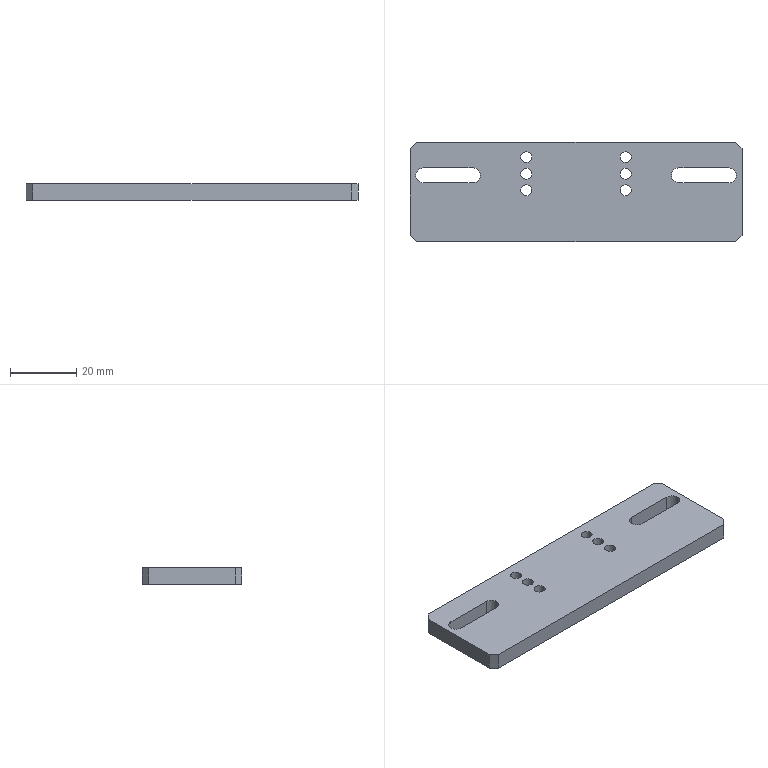Part | STEP file | 11-FG-SZ01611 | 1 solid | 32 faces | box 100 x 30 x 5 mm | volume 13869 mm3 | cylinder 18 | plane 14 | commonest cylinder face diameters 3.3 x12 4.5 x6
STEP:
#1=CARTESIAN_POINT('',(-28.75,5.,0.));
#2=VERTEX_POINT('',#1);
#3=CARTESIAN_POINT('',(-31.,7.25,0.));
#4=VERTEX_POINT('',#3);
#5=CARTESIAN_POINT('',(-31.,5.,0.));
#6=DIRECTION('',(0.,0.,1.));
#7=DIRECTION('',(1.,0.,0.));
#8=AXIS2_PLACEMENT_3D('',#5,#6,#7);
#9=CIRCLE('',#8,2.25);
#10=EDGE_CURVE('',#2,#4,#9,.T.);
#11=ORIENTED_EDGE('',*,*,#10,.F.);
#12=CARTESIAN_POINT('',(-28.75,5.,5.));
#13=VERTEX_POINT('',#12);
#14=CARTESIAN_POINT('',(-28.75,5.,-39.));
#15=DIRECTION('',(0.,0.,1.));
#16=VECTOR('',#15,1000.);
#17=LINE('',#14,#16);
#18=EDGE_CURVE('',#2,#13,#17,.T.);
#19=ORIENTED_EDGE('',*,*,#18,.T.);
#20=CARTESIAN_POINT('',(-31.,7.25,5.));
#21=VERTEX_POINT('',#20);
#22=CARTESIAN_POINT('',(-31.,5.,5.));
#23=DIRECTION('',(0.,0.,1.));
#24=DIRECTION('',(-1.,0.,0.));
#25=AXIS2_PLACEMENT_3D('',#22,#23,#24);
#26=CIRCLE('',#25,2.25);
#27=EDGE_CURVE('',#13,#21,#26,.T.);
#28=ORIENTED_EDGE('',*,*,#27,.T.);
#29=CARTESIAN_POINT('',(-31.,7.25,-39.));
#30=DIRECTION('',(0.,0.,1.));
#31=VECTOR('',#30,1000.);
#32=LINE('',#29,#31);
#33=EDGE_CURVE('',#4,#21,#32,.T.);
#34=ORIENTED_EDGE('',*,*,#33,.F.);
#35=EDGE_LOOP('',(#11,#19,#28,#34));
#36=FACE_OUTER_BOUND('',#35,.T.);
#37=CARTESIAN_POINT('',(-31.,5.,-39.));
#38=DIRECTION('',(0.,0.,1.));
#39=DIRECTION('',(1.,0.,0.));
#40=AXIS2_PLACEMENT_3D('',#37,#38,#39);
#41=CYLINDRICAL_SURFACE('',#40,2.25);
#42=ADVANCED_FACE('',(#36),#41,.F.);
#43=CARTESIAN_POINT('',(48.25,5.,0.));
#44=VERTEX_POINT('',#43);
#45=CARTESIAN_POINT('',(46.,7.25,0.));
#46=VERTEX_POINT('',#45);
#47=CARTESIAN_POINT('',(46.,5.,0.));
#48=DIRECTION('',(0.,0.,1.));
#49=DIRECTION('',(1.,0.,0.));
#50=AXIS2_PLACEMENT_3D('',#47,#48,#49);
#51=CIRCLE('',#50,2.25);
#52=EDGE_CURVE('',#44,#46,#51,.T.);
#53=ORIENTED_EDGE('',*,*,#52,.F.);
#54=CARTESIAN_POINT('',(48.25,5.,5.));
#55=VERTEX_POINT('',#54);
#56=CARTESIAN_POINT('',(48.25,5.,-39.));
#57=DIRECTION('',(0.,0.,1.));
#58=VECTOR('',#57,1000.);
#59=LINE('',#56,#58);
#60=EDGE_CURVE('',#44,#55,#59,.T.);
#61=ORIENTED_EDGE('',*,*,#60,.T.);
#62=CARTESIAN_POINT('',(46.,7.25,5.));
#63=VERTEX_POINT('',#62);
#64=CARTESIAN_POINT('',(46.,5.,5.));
#65=DIRECTION('',(0.,0.,1.));
#66=DIRECTION('',(1.,0.,0.));
#67=AXIS2_PLACEMENT_3D('',#64,#65,#66);
#68=CIRCLE('',#67,2.25);
#69=EDGE_CURVE('',#55,#63,#68,.T.);
#70=ORIENTED_EDGE('',*,*,#69,.T.);
#71=CARTESIAN_POINT('',(46.,7.25,-39.));
#72=DIRECTION('',(0.,0.,1.));
#73=VECTOR('',#72,1000.);
#74=LINE('',#71,#73);
#75=EDGE_CURVE('',#46,#63,#74,.T.);
#76=ORIENTED_EDGE('',*,*,#75,.F.);
#77=EDGE_LOOP('',(#53,#61,#70,#76));
#78=FACE_OUTER_BOUND('',#77,.T.);
#79=CARTESIAN_POINT('',(46.,5.,-39.));
#80=DIRECTION('',(0.,0.,1.));
#81=DIRECTION('',(1.,0.,0.));
#82=AXIS2_PLACEMENT_3D('',#79,#80,#81);
#83=CYLINDRICAL_SURFACE('',#82,2.25);
#84=ADVANCED_FACE('',(#78),#83,.F.);
#85=CARTESIAN_POINT('',(13.35,10.5,0.));
#86=VERTEX_POINT('',#85);
#87=CARTESIAN_POINT('',(16.65,10.5,0.));
#88=VERTEX_POINT('',#87);
#89=CARTESIAN_POINT('',(15.,10.5,0.));
#90=DIRECTION('',(0.,0.,1.));
#91=DIRECTION('',(1.,0.,0.));
#92=AXIS2_PLACEMENT_3D('',#89,#90,#91);
#93=CIRCLE('',#92,1.65);
#94=EDGE_CURVE('',#86,#88,#93,.T.);
#95=ORIENTED_EDGE('',*,*,#94,.F.);
#96=CARTESIAN_POINT('',(13.35,10.5,5.));
#97=VERTEX_POINT('',#96);
#98=CARTESIAN_POINT('',(13.35,10.5,5.));
#99=DIRECTION('',(0.,0.,1.));
#100=VECTOR('',#99,1000.);
#101=LINE('',#98,#100);
#102=EDGE_CURVE('',#86,#97,#101,.T.);
#103=ORIENTED_EDGE('',*,*,#102,.T.);
#104=CARTESIAN_POINT('',(16.65,10.5,5.));
#105=VERTEX_POINT('',#104);
#106=CARTESIAN_POINT('',(15.,10.5,5.));
#107=DIRECTION('',(0.,0.,1.));
#108=DIRECTION('',(1.,0.,0.));
#109=AXIS2_PLACEMENT_3D('',#106,#107,#108);
#110=CIRCLE('',#109,1.65);
#111=EDGE_CURVE('',#97,#105,#110,.T.);
#112=ORIENTED_EDGE('',*,*,#111,.T.);
#113=CARTESIAN_POINT('',(16.65,10.5,5.));
#114=DIRECTION('',(0.,0.,1.));
#115=VECTOR('',#114,1000.);
#116=LINE('',#113,#115);
#117=EDGE_CURVE('',#88,#105,#116,.T.);
#118=ORIENTED_EDGE('',*,*,#117,.F.);
#119=EDGE_LOOP('',(#95,#103,#112,#118));
#120=FACE_OUTER_BOUND('',#119,.T.);
#121=CARTESIAN_POINT('',(15.,10.5,5.));
#122=DIRECTION('',(0.,0.,1.));
#123=DIRECTION('',(1.,0.,0.));
#124=AXIS2_PLACEMENT_3D('',#121,#122,#123);
#125=CYLINDRICAL_SURFACE('',#124,1.65);
#126=ADVANCED_FACE('',(#120),#125,.F.);
#127=CARTESIAN_POINT('',(-16.65,10.5,0.));
#128=VERTEX_POINT('',#127);
#129=CARTESIAN_POINT('',(-13.35,10.5,0.));
#130=VERTEX_POINT('',#129);
#131=CARTESIAN_POINT('',(-15.,10.5,0.));
#132=DIRECTION('',(0.,0.,1.));
#133=DIRECTION('',(1.,0.,0.));
#134=AXIS2_PLACEMENT_3D('',#131,#132,#133);
#135=CIRCLE('',#134,1.65);
#136=EDGE_CURVE('',#128,#130,#135,.T.);
#137=ORIENTED_EDGE('',*,*,#136,.F.);
#138=CARTESIAN_POINT('',(-16.65,10.5,5.));
#139=VERTEX_POINT('',#138);
#140=CARTESIAN_POINT('',(-16.65,10.5,5.));
#141=DIRECTION('',(0.,0.,1.));
#142=VECTOR('',#141,1000.);
#143=LINE('',#140,#142);
#144=EDGE_CURVE('',#128,#139,#143,.T.);
#145=ORIENTED_EDGE('',*,*,#144,.T.);
#146=CARTESIAN_POINT('',(-13.35,10.5,5.));
#147=VERTEX_POINT('',#146);
#148=CARTESIAN_POINT('',(-15.,10.5,5.));
#149=DIRECTION('',(0.,0.,1.));
#150=DIRECTION('',(1.,0.,0.));
#151=AXIS2_PLACEMENT_3D('',#148,#149,#150);
#152=CIRCLE('',#151,1.65);
#153=EDGE_CURVE('',#139,#147,#152,.T.);
#154=ORIENTED_EDGE('',*,*,#153,.T.);
#155=CARTESIAN_POINT('',(-13.35,10.5,5.));
#156=DIRECTION('',(0.,0.,1.));
#157=VECTOR('',#156,1000.);
#158=LINE('',#155,#157);
#159=EDGE_CURVE('',#130,#147,#158,.T.);
#160=ORIENTED_EDGE('',*,*,#159,.F.);
#161=EDGE_LOOP('',(#137,#145,#154,#160));
#162=FACE_OUTER_BOUND('',#161,.T.);
#163=CARTESIAN_POINT('',(-15.,10.5,5.));
#164=DIRECTION('',(0.,0.,1.));
#165=DIRECTION('',(1.,0.,0.));
#166=AXIS2_PLACEMENT_3D('',#163,#164,#165);
#167=CYLINDRICAL_SURFACE('',#166,1.65);
#168=ADVANCED_FACE('',(#162),#167,.F.);
#169=CARTESIAN_POINT('',(13.35,5.5,0.));
#170=VERTEX_POINT('',#169);
#171=CARTESIAN_POINT('',(16.65,5.5,0.));
#172=VERTEX_POINT('',#171);
#173=CARTESIAN_POINT('',(15.,5.5,0.));
#174=DIRECTION('',(0.,0.,1.));
#175=DIRECTION('',(1.,0.,0.));
#176=AXIS2_PLACEMENT_3D('',#173,#174,#175);
#177=CIRCLE('',#176,1.65);
#178=EDGE_CURVE('',#170,#172,#177,.T.);
#179=ORIENTED_EDGE('',*,*,#178,.F.);
#180=CARTESIAN_POINT('',(13.35,5.5,5.));
#181=VERTEX_POINT('',#180);
#182=CARTESIAN_POINT('',(13.35,5.5,5.));
#183=DIRECTION('',(0.,0.,1.));
#184=VECTOR('',#183,1000.);
#185=LINE('',#182,#184);
#186=EDGE_CURVE('',#170,#181,#185,.T.);
#187=ORIENTED_EDGE('',*,*,#186,.T.);
#188=CARTESIAN_POINT('',(16.65,5.5,5.));
#189=VERTEX_POINT('',#188);
#190=CARTESIAN_POINT('',(15.,5.5,5.));
#191=DIRECTION('',(0.,0.,1.));
#192=DIRECTION('',(1.,0.,0.));
#193=AXIS2_PLACEMENT_3D('',#190,#191,#192);
#194=CIRCLE('',#193,1.65);
#195=EDGE_CURVE('',#181,#189,#194,.T.);
#196=ORIENTED_EDGE('',*,*,#195,.T.);
#197=CARTESIAN_POINT('',(16.65,5.5,5.));
#198=DIRECTION('',(0.,0.,1.));
#199=VECTOR('',#198,1000.);
#200=LINE('',#197,#199);
#201=EDGE_CURVE('',#172,#189,#200,.T.);
#202=ORIENTED_EDGE('',*,*,#201,.F.);
#203=EDGE_LOOP('',(#179,#187,#196,#202));
#204=FACE_OUTER_BOUND('',#203,.T.);
#205=CARTESIAN_POINT('',(15.,5.5,5.));
#206=DIRECTION('',(0.,0.,1.));
#207=DIRECTION('',(1.,0.,0.));
#208=AXIS2_PLACEMENT_3D('',#205,#206,#207);
#209=CYLINDRICAL_SURFACE('',#208,1.65);
#210=ADVANCED_FACE('',(#204),#209,.F.);
#211=CARTESIAN_POINT('',(-16.65,5.5,0.));
#212=VERTEX_POINT('',#211);
#213=CARTESIAN_POINT('',(-13.35,5.5,0.));
#214=VERTEX_POINT('',#213);
#215=CARTESIAN_POINT('',(-15.,5.5,0.));
#216=DIRECTION('',(0.,0.,1.));
#217=DIRECTION('',(1.,0.,0.));
#218=AXIS2_PLACEMENT_3D('',#215,#216,#217);
#219=CIRCLE('',#218,1.65);
#220=EDGE_CURVE('',#212,#214,#219,.T.);
#221=ORIENTED_EDGE('',*,*,#220,.F.);
#222=CARTESIAN_POINT('',(-16.65,5.5,5.));
#223=VERTEX_POINT('',#222);
#224=CARTESIAN_POINT('',(-16.65,5.5,5.));
#225=DIRECTION('',(0.,0.,1.));
#226=VECTOR('',#225,1000.);
#227=LINE('',#224,#226);
#228=EDGE_CURVE('',#212,#223,#227,.T.);
#229=ORIENTED_EDGE('',*,*,#228,.T.);
#230=CARTESIAN_POINT('',(-13.35,5.5,5.));
#231=VERTEX_POINT('',#230);
#232=CARTESIAN_POINT('',(-15.,5.5,5.));
#233=DIRECTION('',(0.,0.,1.));
#234=DIRECTION('',(1.,0.,0.));
#235=AXIS2_PLACEMENT_3D('',#232,#233,#234);
#236=CIRCLE('',#235,1.65);
#237=EDGE_CURVE('',#223,#231,#236,.T.);
#238=ORIENTED_EDGE('',*,*,#237,.T.);
#239=CARTESIAN_POINT('',(-13.35,5.5,5.));
#240=DIRECTION('',(0.,0.,1.));
#241=VECTOR('',#240,1000.);
#242=LINE('',#239,#241);
#243=EDGE_CURVE('',#214,#231,#242,.T.);
#244=ORIENTED_EDGE('',*,*,#243,.F.);
#245=EDGE_LOOP('',(#221,#229,#238,#244));
#246=FACE_OUTER_BOUND('',#245,.T.);
#247=CARTESIAN_POINT('',(-15.,5.5,5.));
#248=DIRECTION('',(0.,0.,1.));
#249=DIRECTION('',(1.,0.,0.));
#250=AXIS2_PLACEMENT_3D('',#247,#248,#249);
#251=CYLINDRICAL_SURFACE('',#250,1.65);
#252=ADVANCED_FACE('',(#246),#251,.F.);
#253=CARTESIAN_POINT('',(-16.65,0.5,0.));
#254=VERTEX_POINT('',#253);
#255=CARTESIAN_POINT('',(-13.35,0.5,0.));
#256=VERTEX_POINT('',#255);
#257=CARTESIAN_POINT('',(-15.,0.5,0.));
#258=DIRECTION('',(0.,0.,1.));
#259=DIRECTION('',(1.,0.,0.));
#260=AXIS2_PLACEMENT_3D('',#257,#258,#259);
#261=CIRCLE('',#260,1.65);
#262=EDGE_CURVE('',#254,#256,#261,.T.);
#263=ORIENTED_EDGE('',*,*,#262,.F.);
#264=CARTESIAN_POINT('',(-16.65,0.5,5.));
#265=VERTEX_POINT('',#264);
#266=CARTESIAN_POINT('',(-16.65,0.5,5.));
#267=DIRECTION('',(0.,0.,1.));
#268=VECTOR('',#267,1000.);
#269=LINE('',#266,#268);
#270=EDGE_CURVE('',#254,#265,#269,.T.);
#271=ORIENTED_EDGE('',*,*,#270,.T.);
#272=CARTESIAN_POINT('',(-13.35,0.5,5.));
#273=VERTEX_POINT('',#272);
#274=CARTESIAN_POINT('',(-15.,0.5,5.));
#275=DIRECTION('',(0.,0.,1.));
#276=DIRECTION('',(1.,0.,0.));
#277=AXIS2_PLACEMENT_3D('',#274,#275,#276);
#278=CIRCLE('',#277,1.65);
#279=EDGE_CURVE('',#265,#273,#278,.T.);
#280=ORIENTED_EDGE('',*,*,#279,.T.);
#281=CARTESIAN_POINT('',(-13.35,0.5,5.));
#282=DIRECTION('',(0.,0.,1.));
#283=VECTOR('',#282,1000.);
#284=LINE('',#281,#283);
#285=EDGE_CURVE('',#256,#273,#284,.T.);
#286=ORIENTED_EDGE('',*,*,#285,.F.);
#287=EDGE_LOOP('',(#263,#271,#280,#286));
#288=FACE_OUTER_BOUND('',#287,.T.);
#289=CARTESIAN_POINT('',(-15.,0.5,5.));
#290=DIRECTION('',(0.,0.,1.));
#291=DIRECTION('',(1.,0.,0.));
#292=AXIS2_PLACEMENT_3D('',#289,#290,#291);
#293=CYLINDRICAL_SURFACE('',#292,1.65);
#294=ADVANCED_FACE('',(#288),#293,.F.);
#295=CARTESIAN_POINT('',(13.35,0.5,0.));
#296=VERTEX_POINT('',#295);
#297=CARTESIAN_POINT('',(16.65,0.5,0.));
#298=VERTEX_POINT('',#297);
#299=CARTESIAN_POINT('',(15.,0.5,0.));
#300=DIRECTION('',(0.,0.,1.));
#301=DIRECTION('',(1.,0.,0.));
#302=AXIS2_PLACEMENT_3D('',#299,#300,#301);
#303=CIRCLE('',#302,1.65);
#304=EDGE_CURVE('',#296,#298,#303,.T.);
#305=ORIENTED_EDGE('',*,*,#304,.F.);
#306=CARTESIAN_POINT('',(13.35,0.5,5.));
#307=VERTEX_POINT('',#306);
#308=CARTESIAN_POINT('',(13.35,0.5,5.));
#309=DIRECTION('',(0.,0.,1.));
#310=VECTOR('',#309,1000.);
#311=LINE('',#308,#310);
#312=EDGE_CURVE('',#296,#307,#311,.T.);
#313=ORIENTED_EDGE('',*,*,#312,.T.);
#314=CARTESIAN_POINT('',(16.65,0.5,5.));
#315=VERTEX_POINT('',#314);
#316=CARTESIAN_POINT('',(15.,0.5,5.));
#317=DIRECTION('',(0.,0.,1.));
#318=DIRECTION('',(1.,0.,0.));
#319=AXIS2_PLACEMENT_3D('',#316,#317,#318);
#320=CIRCLE('',#319,1.65);
#321=EDGE_CURVE('',#307,#315,#320,.T.);
#322=ORIENTED_EDGE('',*,*,#321,.T.);
#323=CARTESIAN_POINT('',(16.65,0.5,5.));
#324=DIRECTION('',(0.,0.,1.));
#325=VECTOR('',#324,1000.);
#326=LINE('',#323,#325);
#327=EDGE_CURVE('',#298,#315,#326,.T.);
#328=ORIENTED_EDGE('',*,*,#327,.F.);
#329=EDGE_LOOP('',(#305,#313,#322,#328));
#330=FACE_OUTER_BOUND('',#329,.T.);
#331=CARTESIAN_POINT('',(15.,0.5,5.));
#332=DIRECTION('',(0.,0.,1.));
#333=DIRECTION('',(1.,0.,0.));
#334=AXIS2_PLACEMENT_3D('',#331,#332,#333);
#335=CYLINDRICAL_SURFACE('',#334,1.65);
#336=ADVANCED_FACE('',(#330),#335,.F.);
#337=CARTESIAN_POINT('',(50.,-13.,5.));
#338=VERTEX_POINT('',#337);
#339=CARTESIAN_POINT('',(50.,13.,5.));
#340=VERTEX_POINT('',#339);
#341=CARTESIAN_POINT('',(50.,15.,5.));
#342=DIRECTION('',(0.,1.,0.));
#343=VECTOR('',#342,1000.);
#344=LINE('',#341,#343);
#345=EDGE_CURVE('',#338,#340,#344,.T.);
#346=ORIENTED_EDGE('',*,*,#345,.F.);
#347=CARTESIAN_POINT('',(50.,-13.,0.));
#348=VERTEX_POINT('',#347);
#349=CARTESIAN_POINT('',(50.,-13.,5.));
#350=DIRECTION('',(0.,0.,-1.));
#351=VECTOR('',#350,1000.);
#352=LINE('',#349,#351);
#353=EDGE_CURVE('',#338,#348,#352,.T.);
#354=ORIENTED_EDGE('',*,*,#353,.T.);
#355=CARTESIAN_POINT('',(50.,13.,0.));
#356=VERTEX_POINT('',#355);
#357=CARTESIAN_POINT('',(50.,15.,0.));
#358=DIRECTION('',(0.,1.,0.));
#359=VECTOR('',#358,1000.);
#360=LINE('',#357,#359);
#361=EDGE_CURVE('',#348,#356,#360,.T.);
#362=ORIENTED_EDGE('',*,*,#361,.T.);
#363=CARTESIAN_POINT('',(50.,13.,5.));
#364=DIRECTION('',(0.,0.,1.));
#365=VECTOR('',#364,1000.);
#366=LINE('',#363,#365);
#367=EDGE_CURVE('',#356,#340,#366,.T.);
#368=ORIENTED_EDGE('',*,*,#367,.T.);
#369=EDGE_LOOP('',(#346,#354,#362,#368));
#370=FACE_OUTER_BOUND('',#369,.T.);
#371=CARTESIAN_POINT('',(50.,15.,5.));
#372=DIRECTION('',(-1.,0.,0.));
#373=DIRECTION('',(0.,-1.,0.));
#374=AXIS2_PLACEMENT_3D('',#371,#372,#373);
#375=PLANE('',#374);
#376=ADVANCED_FACE('',(#370),#375,.F.);
#377=CARTESIAN_POINT('',(48.,15.,0.));
#378=VERTEX_POINT('',#377);
#379=CARTESIAN_POINT('',(-48.,15.,0.));
#380=VERTEX_POINT('',#379);
#381=CARTESIAN_POINT('',(-50.,15.,0.));
#382=DIRECTION('',(-1.,0.,0.));
#383=VECTOR('',#382,1000.);
#384=LINE('',#381,#383);
#385=EDGE_CURVE('',#378,#380,#384,.T.);
#386=ORIENTED_EDGE('',*,*,#385,.T.);
#387=CARTESIAN_POINT('',(-48.,15.,5.));
#388=VERTEX_POINT('',#387);
#389=CARTESIAN_POINT('',(-48.,15.,5.));
#390=DIRECTION('',(0.,0.,1.));
#391=VECTOR('',#390,1000.);
#392=LINE('',#389,#391);
#393=EDGE_CURVE('',#380,#388,#392,.T.);
#394=ORIENTED_EDGE('',*,*,#393,.T.);
#395=CARTESIAN_POINT('',(48.,15.,5.));
#396=VERTEX_POINT('',#395);
#397=CARTESIAN_POINT('',(-50.,15.,5.));
#398=DIRECTION('',(-1.,0.,0.));
#399=VECTOR('',#398,1000.);
#400=LINE('',#397,#399);
#401=EDGE_CURVE('',#396,#388,#400,.T.);
#402=ORIENTED_EDGE('',*,*,#401,.F.);
#403=CARTESIAN_POINT('',(48.,15.,5.));
#404=DIRECTION('',(0.,0.,-1.));
#405=VECTOR('',#404,1000.);
#406=LINE('',#403,#405);
#407=EDGE_CURVE('',#396,#378,#406,.T.);
#408=ORIENTED_EDGE('',*,*,#407,.T.);
#409=EDGE_LOOP('',(#386,#394,#402,#408));
#410=FACE_OUTER_BOUND('',#409,.T.);
#411=CARTESIAN_POINT('',(-50.,15.,5.));
#412=DIRECTION('',(0.,-1.,0.));
#413=DIRECTION('',(0.,0.,-1.));
#414=AXIS2_PLACEMENT_3D('',#411,#412,#413);
#415=PLANE('',#414);
#416=ADVANCED_FACE('',(#410),#415,.F.);
#417=CARTESIAN_POINT('',(-50.,13.,0.));
#418=VERTEX_POINT('',#417);
#419=CARTESIAN_POINT('',(-50.,-13.,0.));
#420=VERTEX_POINT('',#419);
#421=CARTESIAN_POINT('',(-50.,15.,0.));
#422=DIRECTION('',(0.,-1.,0.));
#423=VECTOR('',#422,1000.);
#424=LINE('',#421,#423);
#425=EDGE_CURVE('',#418,#420,#424,.T.);
#426=ORIENTED_EDGE('',*,*,#425,.T.);
#427=CARTESIAN_POINT('',(-50.,-13.,5.));
#428=VERTEX_POINT('',#427);
#429=CARTESIAN_POINT('',(-50.,-13.,5.));
#430=DIRECTION('',(0.,0.,1.));
#431=VECTOR('',#430,1000.);
#432=LINE('',#429,#431);
#433=EDGE_CURVE('',#420,#428,#432,.T.);
#434=ORIENTED_EDGE('',*,*,#433,.T.);
#435=CARTESIAN_POINT('',(-50.,13.,5.));
#436=VERTEX_POINT('',#435);
#437=CARTESIAN_POINT('',(-50.,15.,5.));
#438=DIRECTION('',(0.,-1.,0.));
#439=VECTOR('',#438,1000.);
#440=LINE('',#437,#439);
#441=EDGE_CURVE('',#436,#428,#440,.T.);
#442=ORIENTED_EDGE('',*,*,#441,.F.);
#443=CARTESIAN_POINT('',(-50.,13.,5.));
#444=DIRECTION('',(0.,0.,-1.));
#445=VECTOR('',#444,1000.);
#446=LINE('',#443,#445);
#447=EDGE_CURVE('',#436,#418,#446,.T.);
#448=ORIENTED_EDGE('',*,*,#447,.T.);
#449=EDGE_LOOP('',(#426,#434,#442,#448));
#450=FACE_OUTER_BOUND('',#449,.T.);
#451=CARTESIAN_POINT('',(-50.,15.,5.));
#452=DIRECTION('',(1.,0.,0.));
#453=DIRECTION('',(0.,0.,-1.));
#454=AXIS2_PLACEMENT_3D('',#451,#452,#453);
#455=PLANE('',#454);
#456=ADVANCED_FACE('',(#450),#455,.F.);
#457=CARTESIAN_POINT('',(-48.,-15.,5.));
#458=VERTEX_POINT('',#457);
#459=CARTESIAN_POINT('',(48.,-15.,5.));
#460=VERTEX_POINT('',#459);
#461=CARTESIAN_POINT('',(-50.,-15.,5.));
#462=DIRECTION('',(1.,0.,0.));
#463=VECTOR('',#462,1000.);
#464=LINE('',#461,#463);
#465=EDGE_CURVE('',#458,#460,#464,.T.);
#466=ORIENTED_EDGE('',*,*,#465,.F.);
#467=CARTESIAN_POINT('',(-48.,-15.,0.));
#468=VERTEX_POINT('',#467);
#469=CARTESIAN_POINT('',(-48.,-15.,5.));
#470=DIRECTION('',(0.,0.,-1.));
#471=VECTOR('',#470,1000.);
#472=LINE('',#469,#471);
#473=EDGE_CURVE('',#458,#468,#472,.T.);
#474=ORIENTED_EDGE('',*,*,#473,.T.);
#475=CARTESIAN_POINT('',(48.,-15.,0.));
#476=VERTEX_POINT('',#475);
#477=CARTESIAN_POINT('',(-50.,-15.,0.));
#478=DIRECTION('',(1.,0.,0.));
#479=VECTOR('',#478,1000.);
#480=LINE('',#477,#479);
#481=EDGE_CURVE('',#468,#476,#480,.T.);
#482=ORIENTED_EDGE('',*,*,#481,.T.);
#483=CARTESIAN_POINT('',(48.,-15.,5.));
#484=DIRECTION('',(0.,0.,1.));
#485=VECTOR('',#484,1000.);
#486=LINE('',#483,#485);
#487=EDGE_CURVE('',#476,#460,#486,.T.);
#488=ORIENTED_EDGE('',*,*,#487,.T.);
#489=EDGE_LOOP('',(#466,#474,#482,#488));
#490=FACE_OUTER_BOUND('',#489,.T.);
#491=CARTESIAN_POINT('',(-50.,-15.,5.));
#492=DIRECTION('',(0.,1.,0.));
#493=DIRECTION('',(0.,0.,1.));
#494=AXIS2_PLACEMENT_3D('',#491,#492,#493);
#495=PLANE('',#494);
#496=ADVANCED_FACE('',(#490),#495,.F.);
#497=CARTESIAN_POINT('',(-46.,7.25,5.));
#498=VERTEX_POINT('',#497);
#499=CARTESIAN_POINT('',(-46.,2.75,5.));
#500=VERTEX_POINT('',#499);
#501=CARTESIAN_POINT('',(-46.,5.,5.));
#502=DIRECTION('',(0.,0.,1.));
#503=DIRECTION('',(-1.,0.,0.));
#504=AXIS2_PLACEMENT_3D('',#501,#502,#503);
#505=CIRCLE('',#504,2.25);
#506=EDGE_CURVE('',#498,#500,#505,.T.);
#507=ORIENTED_EDGE('',*,*,#506,.F.);
#508=CARTESIAN_POINT('',(-46.,7.25,5.));
#509=DIRECTION('',(-1.,0.,0.));
#510=VECTOR('',#509,1000.);
#511=LINE('',#508,#510);
#512=EDGE_CURVE('',#21,#498,#511,.T.);
#513=ORIENTED_EDGE('',*,*,#512,.F.);
#514=ORIENTED_EDGE('',*,*,#27,.F.);
#515=CARTESIAN_POINT('',(-31.,2.75,5.));
#516=VERTEX_POINT('',#515);
#517=CARTESIAN_POINT('',(-31.,5.,5.));
#518=DIRECTION('',(0.,0.,1.));
#519=DIRECTION('',(-1.,0.,0.));
#520=AXIS2_PLACEMENT_3D('',#517,#518,#519);
#521=CIRCLE('',#520,2.25);
#522=EDGE_CURVE('',#516,#13,#521,.T.);
#523=ORIENTED_EDGE('',*,*,#522,.F.);
#524=CARTESIAN_POINT('',(-46.,2.75,5.));
#525=DIRECTION('',(1.,0.,0.));
#526=VECTOR('',#525,1000.);
#527=LINE('',#524,#526);
#528=EDGE_CURVE('',#500,#516,#527,.T.);
#529=ORIENTED_EDGE('',*,*,#528,.F.);
#530=EDGE_LOOP('',(#507,#513,#514,#523,#529));
#531=FACE_BOUND('',#530,.T.);
#532=CARTESIAN_POINT('',(46.,2.75,5.));
#533=VERTEX_POINT('',#532);
#534=CARTESIAN_POINT('',(46.,5.,5.));
#535=DIRECTION('',(0.,0.,1.));
#536=DIRECTION('',(1.,0.,0.));
#537=AXIS2_PLACEMENT_3D('',#534,#535,#536);
#538=CIRCLE('',#537,2.25);
#539=EDGE_CURVE('',#533,#55,#538,.T.);
#540=ORIENTED_EDGE('',*,*,#539,.F.);
#541=CARTESIAN_POINT('',(31.,2.75,5.));
#542=VERTEX_POINT('',#541);
#543=CARTESIAN_POINT('',(46.,2.75,5.));
#544=DIRECTION('',(1.,0.,0.));
#545=VECTOR('',#544,1000.);
#546=LINE('',#543,#545);
#547=EDGE_CURVE('',#542,#533,#546,.T.);
#548=ORIENTED_EDGE('',*,*,#547,.F.);
#549=CARTESIAN_POINT('',(31.,7.25,5.));
#550=VERTEX_POINT('',#549);
#551=CARTESIAN_POINT('',(31.,5.,5.));
#552=DIRECTION('',(0.,0.,1.));
#553=DIRECTION('',(1.,0.,0.));
#554=AXIS2_PLACEMENT_3D('',#551,#552,#553);
#555=CIRCLE('',#554,2.25);
#556=EDGE_CURVE('',#550,#542,#555,.T.);
#557=ORIENTED_EDGE('',*,*,#556,.F.);
#558=CARTESIAN_POINT('',(46.,7.25,5.));
#559=DIRECTION('',(-1.,0.,0.));
#560=VECTOR('',#559,1000.);
#561=LINE('',#558,#560);
#562=EDGE_CURVE('',#63,#550,#561,.T.);
#563=ORIENTED_EDGE('',*,*,#562,.F.);
#564=ORIENTED_EDGE('',*,*,#69,.F.);
#565=EDGE_LOOP('',(#540,#548,#557,#563,#564));
#566=FACE_BOUND('',#565,.T.);
#567=CARTESIAN_POINT('',(15.,10.5,5.));
#568=DIRECTION('',(0.,0.,1.));
#569=DIRECTION('',(1.,0.,0.));
#570=AXIS2_PLACEMENT_3D('',#567,#568,#569);
#571=CIRCLE('',#570,1.65);
#572=EDGE_CURVE('',#105,#97,#571,.T.);
#573=ORIENTED_EDGE('',*,*,#572,.F.);
#574=ORIENTED_EDGE('',*,*,#111,.F.);
#575=EDGE_LOOP('',(#573,#574));
#576=FACE_BOUND('',#575,.T.);
#577=CARTESIAN_POINT('',(-15.,10.5,5.));
#578=DIRECTION('',(0.,0.,1.));
#579=DIRECTION('',(1.,0.,0.));
#580=AXIS2_PLACEMENT_3D('',#577,#578,#579);
#581=CIRCLE('',#580,1.65);
#582=EDGE_CURVE('',#147,#139,#581,.T.);
#583=ORIENTED_EDGE('',*,*,#582,.F.);
#584=ORIENTED_EDGE('',*,*,#153,.F.);
#585=EDGE_LOOP('',(#583,#584));
#586=FACE_BOUND('',#585,.T.);
#587=CARTESIAN_POINT('',(15.,5.5,5.));
#588=DIRECTION('',(0.,0.,1.));
#589=DIRECTION('',(1.,0.,0.));
#590=AXIS2_PLACEMENT_3D('',#587,#588,#589);
#591=CIRCLE('',#590,1.65);
#592=EDGE_CURVE('',#189,#181,#591,.T.);
#593=ORIENTED_EDGE('',*,*,#592,.F.);
#594=ORIENTED_EDGE('',*,*,#195,.F.);
#595=EDGE_LOOP('',(#593,#594));
#596=FACE_BOUND('',#595,.T.);
#597=CARTESIAN_POINT('',(-15.,5.5,5.));
#598=DIRECTION('',(0.,0.,1.));
#599=DIRECTION('',(1.,0.,0.));
#600=AXIS2_PLACEMENT_3D('',#597,#598,#599);
#601=CIRCLE('',#600,1.65);
#602=EDGE_CURVE('',#231,#223,#601,.T.);
#603=ORIENTED_EDGE('',*,*,#602,.F.);
#604=ORIENTED_EDGE('',*,*,#237,.F.);
#605=EDGE_LOOP('',(#603,#604));
#606=FACE_BOUND('',#605,.T.);
#607=CARTESIAN_POINT('',(-15.,0.5,5.));
#608=DIRECTION('',(0.,0.,1.));
#609=DIRECTION('',(1.,0.,0.));
#610=AXIS2_PLACEMENT_3D('',#607,#608,#609);
#611=CIRCLE('',#610,1.65);
#612=EDGE_CURVE('',#273,#265,#611,.T.);
#613=ORIENTED_EDGE('',*,*,#612,.F.);
#614=ORIENTED_EDGE('',*,*,#279,.F.);
#615=EDGE_LOOP('',(#613,#614));
#616=FACE_BOUND('',#615,.T.);
#617=CARTESIAN_POINT('',(15.,0.5,5.));
#618=DIRECTION('',(0.,0.,1.));
#619=DIRECTION('',(1.,0.,0.));
#620=AXIS2_PLACEMENT_3D('',#617,#618,#619);
#621=CIRCLE('',#620,1.65);
#622=EDGE_CURVE('',#315,#307,#621,.T.);
#623=ORIENTED_EDGE('',*,*,#622,.F.);
#624=ORIENTED_EDGE('',*,*,#321,.F.);
#625=EDGE_LOOP('',(#623,#624));
#626=FACE_BOUND('',#625,.T.);
#627=ORIENTED_EDGE('',*,*,#441,.T.);
#628=CARTESIAN_POINT('',(-31.5,-31.5,5.));
#629=DIRECTION('',(0.7071,-0.7071,0.));
#630=VECTOR('',#629,1000.);
#631=LINE('',#628,#630);
#632=EDGE_CURVE('',#428,#458,#631,.T.);
#633=ORIENTED_EDGE('',*,*,#632,.T.);
#634=ORIENTED_EDGE('',*,*,#465,.T.);
#635=CARTESIAN_POINT('',(31.5,-31.5,5.));
#636=DIRECTION('',(0.7071,0.7071,0.));
#637=VECTOR('',#636,1000.);
#638=LINE('',#635,#637);
#639=EDGE_CURVE('',#460,#338,#638,.T.);
#640=ORIENTED_EDGE('',*,*,#639,.T.);
#641=ORIENTED_EDGE('',*,*,#345,.T.);
#642=CARTESIAN_POINT('',(31.5,31.5,5.));
#643=DIRECTION('',(-0.7071,0.7071,0.));
#644=VECTOR('',#643,1000.);
#645=LINE('',#642,#644);
#646=EDGE_CURVE('',#340,#396,#645,.T.);
#647=ORIENTED_EDGE('',*,*,#646,.T.);
#648=ORIENTED_EDGE('',*,*,#401,.T.);
#649=CARTESIAN_POINT('',(-31.5,31.5,5.));
#650=DIRECTION('',(-0.7071,-0.7071,0.));
#651=VECTOR('',#650,1000.);
#652=LINE('',#649,#651);
#653=EDGE_CURVE('',#388,#436,#652,.T.);
#654=ORIENTED_EDGE('',*,*,#653,.T.);
#655=EDGE_LOOP('',(#627,#633,#634,#640,#641,#647,#648,#654));
#656=FACE_OUTER_BOUND('',#655,.T.);
#657=CARTESIAN_POINT('',(0.,0.,5.));
#658=DIRECTION('',(0.,0.,1.));
#659=DIRECTION('',(1.,0.,0.));
#660=AXIS2_PLACEMENT_3D('',#657,#658,#659);
#661=PLANE('',#660);
#662=ADVANCED_FACE('',(#531,#566,#576,#586,#596,#606,#616,#626,#656),#661,.T.);
#663=CARTESIAN_POINT('',(-46.,7.25,0.));
#664=VERTEX_POINT('',#663);
#665=CARTESIAN_POINT('',(0.,7.25,0.));
#666=DIRECTION('',(-1.,0.,0.));
#667=VECTOR('',#666,1000.);
#668=LINE('',#665,#667);
#669=EDGE_CURVE('',#4,#664,#668,.T.);
#670=ORIENTED_EDGE('',*,*,#669,.T.);
#671=CARTESIAN_POINT('',(-46.,2.75,0.));
#672=VERTEX_POINT('',#671);
#673=CARTESIAN_POINT('',(-46.,5.,0.));
#674=DIRECTION('',(0.,0.,1.));
#675=DIRECTION('',(1.,0.,0.));
#676=AXIS2_PLACEMENT_3D('',#673,#674,#675);
#677=CIRCLE('',#676,2.25);
#678=EDGE_CURVE('',#664,#672,#677,.T.);
#679=ORIENTED_EDGE('',*,*,#678,.T.);
#680=CARTESIAN_POINT('',(-31.,2.75,0.));
#681=VERTEX_POINT('',#680);
#682=CARTESIAN_POINT('',(0.,2.75,0.));
#683=DIRECTION('',(1.,0.,0.));
#684=VECTOR('',#683,1000.);
#685=LINE('',#682,#684);
#686=EDGE_CURVE('',#672,#681,#685,.T.);
#687=ORIENTED_EDGE('',*,*,#686,.T.);
#688=CARTESIAN_POINT('',(-31.,5.,0.));
#689=DIRECTION('',(0.,0.,1.));
#690=DIRECTION('',(1.,0.,0.));
#691=AXIS2_PLACEMENT_3D('',#688,#689,#690);
#692=CIRCLE('',#691,2.25);
#693=EDGE_CURVE('',#681,#2,#692,.T.);
#694=ORIENTED_EDGE('',*,*,#693,.T.);
#695=ORIENTED_EDGE('',*,*,#10,.T.);
#696=EDGE_LOOP('',(#670,#679,#687,#694,#695));
#697=FACE_BOUND('',#696,.T.);
#698=CARTESIAN_POINT('',(31.,2.75,0.));
#699=VERTEX_POINT('',#698);
#700=CARTESIAN_POINT('',(46.,2.75,0.));
#701=VERTEX_POINT('',#700);
#702=CARTESIAN_POINT('',(0.,2.75,0.));
#703=DIRECTION('',(1.,0.,0.));
#704=VECTOR('',#703,1000.);
#705=LINE('',#702,#704);
#706=EDGE_CURVE('',#699,#701,#705,.T.);
#707=ORIENTED_EDGE('',*,*,#706,.T.);
#708=CARTESIAN_POINT('',(46.,5.,0.));
#709=DIRECTION('',(0.,0.,1.));
#710=DIRECTION('',(1.,0.,0.));
#711=AXIS2_PLACEMENT_3D('',#708,#709,#710);
#712=CIRCLE('',#711,2.25);
#713=EDGE_CURVE('',#701,#44,#712,.T.);
#714=ORIENTED_EDGE('',*,*,#713,.T.);
#715=ORIENTED_EDGE('',*,*,#52,.T.);
#716=CARTESIAN_POINT('',(31.,7.25,0.));
#717=VERTEX_POINT('',#716);
#718=CARTESIAN_POINT('',(0.,7.25,0.));
#719=DIRECTION('',(-1.,0.,0.));
#720=VECTOR('',#719,1000.);
#721=LINE('',#718,#720);
#722=EDGE_CURVE('',#46,#717,#721,.T.);
#723=ORIENTED_EDGE('',*,*,#722,.T.);
#724=CARTESIAN_POINT('',(31.,5.,0.));
#725=DIRECTION('',(0.,0.,1.));
#726=DIRECTION('',(1.,0.,0.));
#727=AXIS2_PLACEMENT_3D('',#724,#725,#726);
#728=CIRCLE('',#727,2.25);
#729=EDGE_CURVE('',#717,#699,#728,.T.);
#730=ORIENTED_EDGE('',*,*,#729,.T.);
#731=EDGE_LOOP('',(#707,#714,#715,#723,#730));
#732=FACE_BOUND('',#731,.T.);
#733=CARTESIAN_POINT('',(15.,10.5,0.));
#734=DIRECTION('',(0.,0.,1.));
#735=DIRECTION('',(1.,0.,0.));
#736=AXIS2_PLACEMENT_3D('',#733,#734,#735);
#737=CIRCLE('',#736,1.65);
#738=EDGE_CURVE('',#88,#86,#737,.T.);
#739=ORIENTED_EDGE('',*,*,#738,.T.);
#740=ORIENTED_EDGE('',*,*,#94,.T.);
#741=EDGE_LOOP('',(#739,#740));
#742=FACE_BOUND('',#741,.T.);
#743=CARTESIAN_POINT('',(-15.,10.5,0.));
#744=DIRECTION('',(0.,0.,1.));
#745=DIRECTION('',(1.,0.,0.));
#746=AXIS2_PLACEMENT_3D('',#743,#744,#745);
#747=CIRCLE('',#746,1.65);
#748=EDGE_CURVE('',#130,#128,#747,.T.);
#749=ORIENTED_EDGE('',*,*,#748,.T.);
#750=ORIENTED_EDGE('',*,*,#136,.T.);
#751=EDGE_LOOP('',(#749,#750));
#752=FACE_BOUND('',#751,.T.);
#753=CARTESIAN_POINT('',(15.,5.5,0.));
#754=DIRECTION('',(0.,0.,1.));
#755=DIRECTION('',(1.,0.,0.));
#756=AXIS2_PLACEMENT_3D('',#753,#754,#755);
#757=CIRCLE('',#756,1.65);
#758=EDGE_CURVE('',#172,#170,#757,.T.);
#759=ORIENTED_EDGE('',*,*,#758,.T.);
#760=ORIENTED_EDGE('',*,*,#178,.T.);
#761=EDGE_LOOP('',(#759,#760));
#762=FACE_BOUND('',#761,.T.);
#763=CARTESIAN_POINT('',(-15.,5.5,0.));
#764=DIRECTION('',(0.,0.,1.));
#765=DIRECTION('',(1.,0.,0.));
#766=AXIS2_PLACEMENT_3D('',#763,#764,#765);
#767=CIRCLE('',#766,1.65);
#768=EDGE_CURVE('',#214,#212,#767,.T.);
#769=ORIENTED_EDGE('',*,*,#768,.T.);
#770=ORIENTED_EDGE('',*,*,#220,.T.);
#771=EDGE_LOOP('',(#769,#770));
#772=FACE_BOUND('',#771,.T.);
#773=CARTESIAN_POINT('',(-15.,0.5,0.));
#774=DIRECTION('',(0.,0.,1.));
#775=DIRECTION('',(1.,0.,0.));
#776=AXIS2_PLACEMENT_3D('',#773,#774,#775);
#777=CIRCLE('',#776,1.65);
#778=EDGE_CURVE('',#256,#254,#777,.T.);
#779=ORIENTED_EDGE('',*,*,#778,.T.);
#780=ORIENTED_EDGE('',*,*,#262,.T.);
#781=EDGE_LOOP('',(#779,#780));
#782=FACE_BOUND('',#781,.T.);
#783=CARTESIAN_POINT('',(15.,0.5,0.));
#784=DIRECTION('',(0.,0.,1.));
#785=DIRECTION('',(1.,0.,0.));
#786=AXIS2_PLACEMENT_3D('',#783,#784,#785);
#787=CIRCLE('',#786,1.65);
#788=EDGE_CURVE('',#298,#296,#787,.T.);
#789=ORIENTED_EDGE('',*,*,#788,.T.);
#790=ORIENTED_EDGE('',*,*,#304,.T.);
#791=EDGE_LOOP('',(#789,#790));
#792=FACE_BOUND('',#791,.T.);
#793=ORIENTED_EDGE('',*,*,#481,.F.);
#794=CARTESIAN_POINT('',(-48.,-15.,0.));
#795=DIRECTION('',(-0.7071,0.7071,0.));
#796=VECTOR('',#795,1000.);
#797=LINE('',#794,#796);
#798=EDGE_CURVE('',#468,#420,#797,.T.);
#799=ORIENTED_EDGE('',*,*,#798,.T.);
#800=ORIENTED_EDGE('',*,*,#425,.F.);
#801=CARTESIAN_POINT('',(-50.,13.,0.));
#802=DIRECTION('',(0.7071,0.7071,0.));
#803=VECTOR('',#802,1000.);
#804=LINE('',#801,#803);
#805=EDGE_CURVE('',#418,#380,#804,.T.);
#806=ORIENTED_EDGE('',*,*,#805,.T.);
#807=ORIENTED_EDGE('',*,*,#385,.F.);
#808=CARTESIAN_POINT('',(48.,15.,0.));
#809=DIRECTION('',(0.7071,-0.7071,0.));
#810=VECTOR('',#809,1000.);
#811=LINE('',#808,#810);
#812=EDGE_CURVE('',#378,#356,#811,.T.);
#813=ORIENTED_EDGE('',*,*,#812,.T.);
#814=ORIENTED_EDGE('',*,*,#361,.F.);
#815=CARTESIAN_POINT('',(50.,-13.,0.));
#816=DIRECTION('',(-0.7071,-0.7071,0.));
#817=VECTOR('',#816,1000.);
#818=LINE('',#815,#817);
#819=EDGE_CURVE('',#348,#476,#818,.T.);
#820=ORIENTED_EDGE('',*,*,#819,.T.);
#821=EDGE_LOOP('',(#793,#799,#800,#806,#807,#813,#814,#820));
#822=FACE_OUTER_BOUND('',#821,.T.);
#823=CARTESIAN_POINT('',(0.,0.,0.));
#824=DIRECTION('',(0.,0.,1.));
#825=DIRECTION('',(1.,0.,0.));
#826=AXIS2_PLACEMENT_3D('',#823,#824,#825);
#827=PLANE('',#826);
#828=ADVANCED_FACE('',(#697,#732,#742,#752,#762,#772,#782,#792,#822),#827,.F.);
#829=ORIENTED_EDGE('',*,*,#632,.F.);
#830=ORIENTED_EDGE('',*,*,#433,.F.);
#831=ORIENTED_EDGE('',*,*,#798,.F.);
#832=ORIENTED_EDGE('',*,*,#473,.F.);
#833=EDGE_LOOP('',(#829,#830,#831,#832));
#834=FACE_OUTER_BOUND('',#833,.T.);
#835=CARTESIAN_POINT('',(-48.,-15.,5.));
#836=DIRECTION('',(0.7071,0.7071,0.));
#837=DIRECTION('',(0.,0.,-1.));
#838=AXIS2_PLACEMENT_3D('',#835,#836,#837);
#839=PLANE('',#838);
#840=ADVANCED_FACE('',(#834),#839,.F.);
#841=ORIENTED_EDGE('',*,*,#653,.F.);
#842=ORIENTED_EDGE('',*,*,#393,.F.);
#843=ORIENTED_EDGE('',*,*,#805,.F.);
#844=ORIENTED_EDGE('',*,*,#447,.F.);
#845=EDGE_LOOP('',(#841,#842,#843,#844));
#846=FACE_OUTER_BOUND('',#845,.T.);
#847=CARTESIAN_POINT('',(-50.,13.,5.));
#848=DIRECTION('',(0.7071,-0.7071,0.));
#849=DIRECTION('',(0.,0.,-1.));
#850=AXIS2_PLACEMENT_3D('',#847,#848,#849);
#851=PLANE('',#850);
#852=ADVANCED_FACE('',(#846),#851,.F.);
#853=ORIENTED_EDGE('',*,*,#639,.F.);
#854=ORIENTED_EDGE('',*,*,#487,.F.);
#855=ORIENTED_EDGE('',*,*,#819,.F.);
#856=ORIENTED_EDGE('',*,*,#353,.F.);
#857=EDGE_LOOP('',(#853,#854,#855,#856));
#858=FACE_OUTER_BOUND('',#857,.T.);
#859=CARTESIAN_POINT('',(50.,-13.,5.));
#860=DIRECTION('',(-0.7071,0.7071,0.));
#861=DIRECTION('',(0.,0.,-1.));
#862=AXIS2_PLACEMENT_3D('',#859,#860,#861);
#863=PLANE('',#862);
#864=ADVANCED_FACE('',(#858),#863,.F.);
#865=ORIENTED_EDGE('',*,*,#646,.F.);
#866=ORIENTED_EDGE('',*,*,#367,.F.);
#867=ORIENTED_EDGE('',*,*,#812,.F.);
#868=ORIENTED_EDGE('',*,*,#407,.F.);
#869=EDGE_LOOP('',(#865,#866,#867,#868));
#870=FACE_OUTER_BOUND('',#869,.T.);
#871=CARTESIAN_POINT('',(48.,15.,5.));
#872=DIRECTION('',(-0.7071,-0.7071,0.));
#873=DIRECTION('',(0.,0.,-1.));
#874=AXIS2_PLACEMENT_3D('',#871,#872,#873);
#875=PLANE('',#874);
#876=ADVANCED_FACE('',(#870),#875,.F.);
#877=ORIENTED_EDGE('',*,*,#312,.F.);
#878=ORIENTED_EDGE('',*,*,#788,.F.);
#879=ORIENTED_EDGE('',*,*,#327,.T.);
#880=ORIENTED_EDGE('',*,*,#622,.T.);
#881=EDGE_LOOP('',(#877,#878,#879,#880));
#882=FACE_OUTER_BOUND('',#881,.T.);
#883=CARTESIAN_POINT('',(15.,0.5,5.));
#884=DIRECTION('',(0.,0.,1.));
#885=DIRECTION('',(1.,0.,0.));
#886=AXIS2_PLACEMENT_3D('',#883,#884,#885);
#887=CYLINDRICAL_SURFACE('',#886,1.65);
#888=ADVANCED_FACE('',(#882),#887,.F.);
#889=ORIENTED_EDGE('',*,*,#270,.F.);
#890=ORIENTED_EDGE('',*,*,#778,.F.);
#891=ORIENTED_EDGE('',*,*,#285,.T.);
#892=ORIENTED_EDGE('',*,*,#612,.T.);
#893=EDGE_LOOP('',(#889,#890,#891,#892));
#894=FACE_OUTER_BOUND('',#893,.T.);
#895=CARTESIAN_POINT('',(-15.,0.5,5.));
#896=DIRECTION('',(0.,0.,1.));
#897=DIRECTION('',(1.,0.,0.));
#898=AXIS2_PLACEMENT_3D('',#895,#896,#897);
#899=CYLINDRICAL_SURFACE('',#898,1.65);
#900=ADVANCED_FACE('',(#894),#899,.F.);
#901=ORIENTED_EDGE('',*,*,#228,.F.);
#902=ORIENTED_EDGE('',*,*,#768,.F.);
#903=ORIENTED_EDGE('',*,*,#243,.T.);
#904=ORIENTED_EDGE('',*,*,#602,.T.);
#905=EDGE_LOOP('',(#901,#902,#903,#904));
#906=FACE_OUTER_BOUND('',#905,.T.);
#907=CARTESIAN_POINT('',(-15.,5.5,5.));
#908=DIRECTION('',(0.,0.,1.));
#909=DIRECTION('',(1.,0.,0.));
#910=AXIS2_PLACEMENT_3D('',#907,#908,#909);
#911=CYLINDRICAL_SURFACE('',#910,1.65);
#912=ADVANCED_FACE('',(#906),#911,.F.);
#913=ORIENTED_EDGE('',*,*,#186,.F.);
#914=ORIENTED_EDGE('',*,*,#758,.F.);
#915=ORIENTED_EDGE('',*,*,#201,.T.);
#916=ORIENTED_EDGE('',*,*,#592,.T.);
#917=EDGE_LOOP('',(#913,#914,#915,#916));
#918=FACE_OUTER_BOUND('',#917,.T.);
#919=CARTESIAN_POINT('',(15.,5.5,5.));
#920=DIRECTION('',(0.,0.,1.));
#921=DIRECTION('',(1.,0.,0.));
#922=AXIS2_PLACEMENT_3D('',#919,#920,#921);
#923=CYLINDRICAL_SURFACE('',#922,1.65);
#924=ADVANCED_FACE('',(#918),#923,.F.);
#925=ORIENTED_EDGE('',*,*,#144,.F.);
#926=ORIENTED_EDGE('',*,*,#748,.F.);
#927=ORIENTED_EDGE('',*,*,#159,.T.);
#928=ORIENTED_EDGE('',*,*,#582,.T.);
#929=EDGE_LOOP('',(#925,#926,#927,#928));
#930=FACE_OUTER_BOUND('',#929,.T.);
#931=CARTESIAN_POINT('',(-15.,10.5,5.));
#932=DIRECTION('',(0.,0.,1.));
#933=DIRECTION('',(1.,0.,0.));
#934=AXIS2_PLACEMENT_3D('',#931,#932,#933);
#935=CYLINDRICAL_SURFACE('',#934,1.65);
#936=ADVANCED_FACE('',(#930),#935,.F.);
#937=ORIENTED_EDGE('',*,*,#102,.F.);
#938=ORIENTED_EDGE('',*,*,#738,.F.);
#939=ORIENTED_EDGE('',*,*,#117,.T.);
#940=ORIENTED_EDGE('',*,*,#572,.T.);
#941=EDGE_LOOP('',(#937,#938,#939,#940));
#942=FACE_OUTER_BOUND('',#941,.T.);
#943=CARTESIAN_POINT('',(15.,10.5,5.));
#944=DIRECTION('',(0.,0.,1.));
#945=DIRECTION('',(1.,0.,0.));
#946=AXIS2_PLACEMENT_3D('',#943,#944,#945);
#947=CYLINDRICAL_SURFACE('',#946,1.65);
#948=ADVANCED_FACE('',(#942),#947,.F.);
#949=ORIENTED_EDGE('',*,*,#60,.F.);
#950=ORIENTED_EDGE('',*,*,#713,.F.);
#951=CARTESIAN_POINT('',(46.,2.75,-39.));
#952=DIRECTION('',(0.,0.,1.));
#953=VECTOR('',#952,1000.);
#954=LINE('',#951,#953);
#955=EDGE_CURVE('',#701,#533,#954,.T.);
#956=ORIENTED_EDGE('',*,*,#955,.T.);
#957=ORIENTED_EDGE('',*,*,#539,.T.);
#958=EDGE_LOOP('',(#949,#950,#956,#957));
#959=FACE_OUTER_BOUND('',#958,.T.);
#960=CARTESIAN_POINT('',(46.,5.,-39.));
#961=DIRECTION('',(0.,0.,1.));
#962=DIRECTION('',(1.,0.,0.));
#963=AXIS2_PLACEMENT_3D('',#960,#961,#962);
#964=CYLINDRICAL_SURFACE('',#963,2.25);
#965=ADVANCED_FACE('',(#959),#964,.F.);
#966=CARTESIAN_POINT('',(31.,2.75,-39.));
#967=DIRECTION('',(0.,0.,1.));
#968=VECTOR('',#967,1000.);
#969=LINE('',#966,#968);
#970=EDGE_CURVE('',#699,#542,#969,.T.);
#971=ORIENTED_EDGE('',*,*,#970,.T.);
#972=ORIENTED_EDGE('',*,*,#547,.T.);
#973=ORIENTED_EDGE('',*,*,#955,.F.);
#974=ORIENTED_EDGE('',*,*,#706,.F.);
#975=EDGE_LOOP('',(#971,#972,#973,#974));
#976=FACE_OUTER_BOUND('',#975,.T.);
#977=CARTESIAN_POINT('',(46.,2.75,-39.));
#978=DIRECTION('',(0.,-1.,0.));
#979=DIRECTION('',(1.,0.,0.));
#980=AXIS2_PLACEMENT_3D('',#977,#978,#979);
#981=PLANE('',#980);
#982=ADVANCED_FACE('',(#976),#981,.F.);
#983=CARTESIAN_POINT('',(31.,7.25,-39.));
#984=DIRECTION('',(0.,0.,1.));
#985=VECTOR('',#984,1000.);
#986=LINE('',#983,#985);
#987=EDGE_CURVE('',#717,#550,#986,.T.);
#988=ORIENTED_EDGE('',*,*,#987,.T.);
#989=ORIENTED_EDGE('',*,*,#556,.T.);
#990=ORIENTED_EDGE('',*,*,#970,.F.);
#991=ORIENTED_EDGE('',*,*,#729,.F.);
#992=EDGE_LOOP('',(#988,#989,#990,#991));
#993=FACE_OUTER_BOUND('',#992,.T.);
#994=CARTESIAN_POINT('',(31.,5.,-39.));
#995=DIRECTION('',(0.,0.,1.));
#996=DIRECTION('',(1.,0.,0.));
#997=AXIS2_PLACEMENT_3D('',#994,#995,#996);
#998=CYLINDRICAL_SURFACE('',#997,2.25);
#999=ADVANCED_FACE('',(#993),#998,.F.);
#1000=ORIENTED_EDGE('',*,*,#75,.T.);
#1001=ORIENTED_EDGE('',*,*,#562,.T.);
#1002=ORIENTED_EDGE('',*,*,#987,.F.);
#1003=ORIENTED_EDGE('',*,*,#722,.F.);
#1004=EDGE_LOOP('',(#1000,#1001,#1002,#1003));
#1005=FACE_OUTER_BOUND('',#1004,.T.);
#1006=CARTESIAN_POINT('',(46.,7.25,-39.));
#1007=DIRECTION('',(0.,1.,0.));
#1008=DIRECTION('',(-1.,0.,0.));
#1009=AXIS2_PLACEMENT_3D('',#1006,#1007,#1008);
#1010=PLANE('',#1009);
#1011=ADVANCED_FACE('',(#1005),#1010,.F.);
#1012=CARTESIAN_POINT('',(-46.,7.25,-39.));
#1013=DIRECTION('',(0.,0.,1.));
#1014=VECTOR('',#1013,1000.);
#1015=LINE('',#1012,#1014);
#1016=EDGE_CURVE('',#664,#498,#1015,.T.);
#1017=ORIENTED_EDGE('',*,*,#1016,.T.);
#1018=ORIENTED_EDGE('',*,*,#506,.T.);
#1019=CARTESIAN_POINT('',(-46.,2.75,-39.));
#1020=DIRECTION('',(0.,0.,1.));
#1021=VECTOR('',#1020,1000.);
#1022=LINE('',#1019,#1021);
#1023=EDGE_CURVE('',#672,#500,#1022,.T.);
#1024=ORIENTED_EDGE('',*,*,#1023,.F.);
#1025=ORIENTED_EDGE('',*,*,#678,.F.);
#1026=EDGE_LOOP('',(#1017,#1018,#1024,#1025));
#1027=FACE_OUTER_BOUND('',#1026,.T.);
#1028=CARTESIAN_POINT('',(-46.,5.,-39.));
#1029=DIRECTION('',(0.,0.,1.));
#1030=DIRECTION('',(1.,0.,0.));
#1031=AXIS2_PLACEMENT_3D('',#1028,#1029,#1030);
#1032=CYLINDRICAL_SURFACE('',#1031,2.25);
#1033=ADVANCED_FACE('',(#1027),#1032,.F.);
#1034=ORIENTED_EDGE('',*,*,#33,.T.);
#1035=ORIENTED_EDGE('',*,*,#512,.T.);
#1036=ORIENTED_EDGE('',*,*,#1016,.F.);
#1037=ORIENTED_EDGE('',*,*,#669,.F.);
#1038=EDGE_LOOP('',(#1034,#1035,#1036,#1037));
#1039=FACE_OUTER_BOUND('',#1038,.T.);
#1040=CARTESIAN_POINT('',(-46.,7.25,-39.));
#1041=DIRECTION('',(0.,1.,0.));
#1042=DIRECTION('',(-1.,0.,0.));
#1043=AXIS2_PLACEMENT_3D('',#1040,#1041,#1042);
#1044=PLANE('',#1043);
#1045=ADVANCED_FACE('',(#1039),#1044,.F.);
#1046=ORIENTED_EDGE('',*,*,#18,.F.);
#1047=ORIENTED_EDGE('',*,*,#693,.F.);
#1048=CARTESIAN_POINT('',(-31.,2.75,-39.));
#1049=DIRECTION('',(0.,0.,1.));
#1050=VECTOR('',#1049,1000.);
#1051=LINE('',#1048,#1050);
#1052=EDGE_CURVE('',#681,#516,#1051,.T.);
#1053=ORIENTED_EDGE('',*,*,#1052,.T.);
#1054=ORIENTED_EDGE('',*,*,#522,.T.);
#1055=EDGE_LOOP('',(#1046,#1047,#1053,#1054));
#1056=FACE_OUTER_BOUND('',#1055,.T.);
#1057=CARTESIAN_POINT('',(-31.,5.,-39.));
#1058=DIRECTION('',(0.,0.,1.));
#1059=DIRECTION('',(1.,0.,0.));
#1060=AXIS2_PLACEMENT_3D('',#1057,#1058,#1059);
#1061=CYLINDRICAL_SURFACE('',#1060,2.25);
#1062=ADVANCED_FACE('',(#1056),#1061,.F.);
#1063=ORIENTED_EDGE('',*,*,#1023,.T.);
#1064=ORIENTED_EDGE('',*,*,#528,.T.);
#1065=ORIENTED_EDGE('',*,*,#1052,.F.);
#1066=ORIENTED_EDGE('',*,*,#686,.F.);
#1067=EDGE_LOOP('',(#1063,#1064,#1065,#1066));
#1068=FACE_OUTER_BOUND('',#1067,.T.);
#1069=CARTESIAN_POINT('',(-46.,2.75,-39.));
#1070=DIRECTION('',(0.,-1.,0.));
#1071=DIRECTION('',(1.,0.,0.));
#1072=AXIS2_PLACEMENT_3D('',#1069,#1070,#1071);
#1073=PLANE('',#1072);
#1074=ADVANCED_FACE('',(#1068),#1073,.F.);
#1075=CLOSED_SHELL('',(#42,#84,#126,#168,#210,#252,#294,#336,#376,#416,#456,#496,#662,#828,#840,#852,#864,#876,#888,#900,#912,#924,#936,#948,#965,#982,#999,#1011,#1033,#1045,#1062,#1074));
#1076=MANIFOLD_SOLID_BREP('',#1075);
#1077=CARTESIAN_POINT('',(0.,0.,0.));
#1078=DIRECTION('',(0.,0.,1.));
#1079=DIRECTION('',(1.,0.,0.));
#1080=AXIS2_PLACEMENT_3D('',#1077,#1078,#1079);
#1081=(LENGTH_UNIT()NAMED_UNIT(*)SI_UNIT(.MILLI.,.METRE.));
#1082=UNCERTAINTY_MEASURE_WITH_UNIT(LENGTH_MEASURE(0.00001),#1081,'','');
#1083=(NAMED_UNIT(*)PLANE_ANGLE_UNIT()SI_UNIT($,.RADIAN.));
#1084=(NAMED_UNIT(*)SI_UNIT($,.STERADIAN.)SOLID_ANGLE_UNIT());
#1085=(GEOMETRIC_REPRESENTATION_CONTEXT(3)GLOBAL_UNCERTAINTY_ASSIGNED_CONTEXT((#1082))GLOBAL_UNIT_ASSIGNED_CONTEXT((#1081,#1083,#1084))REPRESENTATION_CONTEXT('',''));
#1086=ADVANCED_BREP_SHAPE_REPRESENTATION('',(#1076,#1080),#1085);